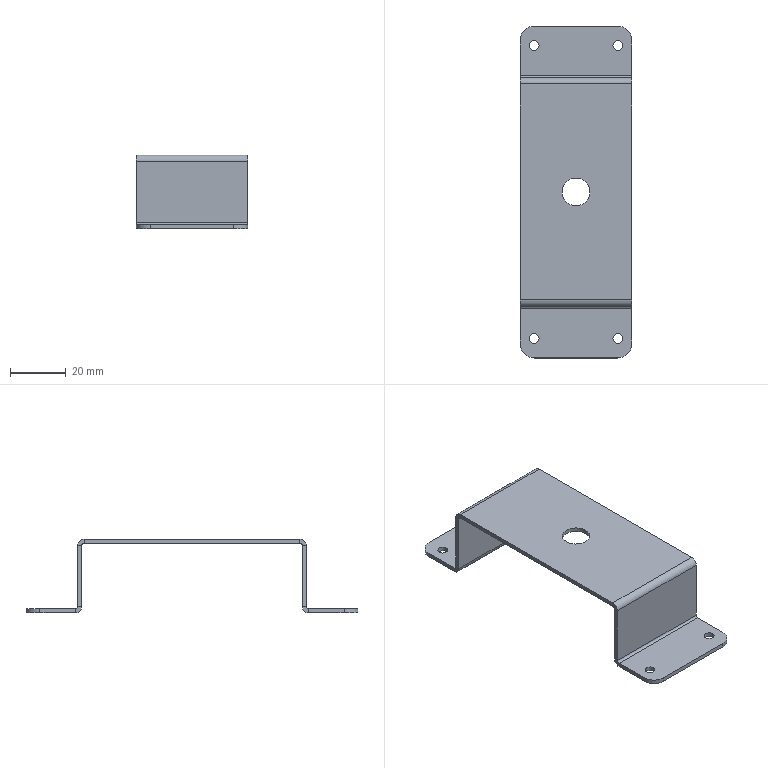Part | SolidWorks | features EdgeFlange 2, ICE 2, Fillet 1, FlatPattern 1, LPattern 1, SMBaseFlange 1, SheetMetal 1 | 1 solid | 52 faces | box 40 x 119 x 26.5 mm | volume 9773 mm3 | plane 30 | cylinder 22 | commonest cylinder face diameters 3.5 x8 10 x6 1.6 x4 4.6 x4
STEP:
#1=CARTESIAN_POINT('',(13.25,52.5,-26.5));
#2=VERTEX_POINT('',#1);
#3=CARTESIAN_POINT('',(16.75,52.5,-26.5));
#4=VERTEX_POINT('',#3);
#5=CARTESIAN_POINT('',(15.,52.5,-26.5));
#6=DIRECTION('',(0.,0.,1.));
#7=DIRECTION('',(1.,0.,0.));
#8=AXIS2_PLACEMENT_3D('',#5,#6,#7);
#9=CIRCLE('',#8,1.75);
#10=EDGE_CURVE('',#2,#4,#9,.T.);
#11=ORIENTED_EDGE('',*,*,#10,.F.);
#12=CARTESIAN_POINT('',(13.25,52.5,-25.));
#13=VERTEX_POINT('',#12);
#14=CARTESIAN_POINT('',(13.25,52.5,-35.));
#15=DIRECTION('',(0.,0.,1.));
#16=VECTOR('',#15,1000.);
#17=LINE('',#14,#16);
#18=EDGE_CURVE('',#2,#13,#17,.T.);
#19=ORIENTED_EDGE('',*,*,#18,.T.);
#20=CARTESIAN_POINT('',(16.75,52.5,-25.));
#21=VERTEX_POINT('',#20);
#22=CARTESIAN_POINT('',(15.,52.5,-25.));
#23=DIRECTION('',(0.,0.,1.));
#24=DIRECTION('',(1.,0.,0.));
#25=AXIS2_PLACEMENT_3D('',#22,#23,#24);
#26=CIRCLE('',#25,1.75);
#27=EDGE_CURVE('',#13,#21,#26,.T.);
#28=ORIENTED_EDGE('',*,*,#27,.T.);
#29=CARTESIAN_POINT('',(16.75,52.5,-35.));
#30=DIRECTION('',(0.,0.,1.));
#31=VECTOR('',#30,1000.);
#32=LINE('',#29,#31);
#33=EDGE_CURVE('',#4,#21,#32,.T.);
#34=ORIENTED_EDGE('',*,*,#33,.F.);
#35=EDGE_LOOP('',(#11,#19,#28,#34));
#36=FACE_OUTER_BOUND('',#35,.T.);
#37=CARTESIAN_POINT('',(15.,52.5,-35.));
#38=DIRECTION('',(0.,0.,1.));
#39=DIRECTION('',(1.,0.,0.));
#40=AXIS2_PLACEMENT_3D('',#37,#38,#39);
#41=CYLINDRICAL_SURFACE('',#40,1.75);
#42=ADVANCED_FACE('',(#36),#41,.F.);
#43=CARTESIAN_POINT('',(-16.75,-52.5,-26.5));
#44=VERTEX_POINT('',#43);
#45=CARTESIAN_POINT('',(-13.25,-52.5,-26.5));
#46=VERTEX_POINT('',#45);
#47=CARTESIAN_POINT('',(-15.,-52.5,-26.5));
#48=DIRECTION('',(0.,0.,1.));
#49=DIRECTION('',(1.,0.,0.));
#50=AXIS2_PLACEMENT_3D('',#47,#48,#49);
#51=CIRCLE('',#50,1.75);
#52=EDGE_CURVE('',#44,#46,#51,.T.);
#53=ORIENTED_EDGE('',*,*,#52,.F.);
#54=CARTESIAN_POINT('',(-16.75,-52.5,-25.));
#55=VERTEX_POINT('',#54);
#56=CARTESIAN_POINT('',(-16.75,-52.5,-35.));
#57=DIRECTION('',(0.,0.,1.));
#58=VECTOR('',#57,1000.);
#59=LINE('',#56,#58);
#60=EDGE_CURVE('',#44,#55,#59,.T.);
#61=ORIENTED_EDGE('',*,*,#60,.T.);
#62=CARTESIAN_POINT('',(-13.25,-52.5,-25.));
#63=VERTEX_POINT('',#62);
#64=CARTESIAN_POINT('',(-15.,-52.5,-25.));
#65=DIRECTION('',(0.,0.,1.));
#66=DIRECTION('',(1.,0.,0.));
#67=AXIS2_PLACEMENT_3D('',#64,#65,#66);
#68=CIRCLE('',#67,1.75);
#69=EDGE_CURVE('',#55,#63,#68,.T.);
#70=ORIENTED_EDGE('',*,*,#69,.T.);
#71=CARTESIAN_POINT('',(-13.25,-52.5,-35.));
#72=DIRECTION('',(0.,0.,1.));
#73=VECTOR('',#72,1000.);
#74=LINE('',#71,#73);
#75=EDGE_CURVE('',#46,#63,#74,.T.);
#76=ORIENTED_EDGE('',*,*,#75,.F.);
#77=EDGE_LOOP('',(#53,#61,#70,#76));
#78=FACE_OUTER_BOUND('',#77,.T.);
#79=CARTESIAN_POINT('',(-15.,-52.5,-35.));
#80=DIRECTION('',(0.,0.,1.));
#81=DIRECTION('',(1.,0.,0.));
#82=AXIS2_PLACEMENT_3D('',#79,#80,#81);
#83=CYLINDRICAL_SURFACE('',#82,1.75);
#84=ADVANCED_FACE('',(#78),#83,.F.);
#85=CARTESIAN_POINT('',(13.25,-52.5,-26.5));
#86=VERTEX_POINT('',#85);
#87=CARTESIAN_POINT('',(16.75,-52.5,-26.5));
#88=VERTEX_POINT('',#87);
#89=CARTESIAN_POINT('',(15.,-52.5,-26.5));
#90=DIRECTION('',(0.,0.,1.));
#91=DIRECTION('',(1.,0.,0.));
#92=AXIS2_PLACEMENT_3D('',#89,#90,#91);
#93=CIRCLE('',#92,1.75);
#94=EDGE_CURVE('',#86,#88,#93,.T.);
#95=ORIENTED_EDGE('',*,*,#94,.F.);
#96=CARTESIAN_POINT('',(13.25,-52.5,-25.));
#97=VERTEX_POINT('',#96);
#98=CARTESIAN_POINT('',(13.25,-52.5,-35.));
#99=DIRECTION('',(0.,0.,1.));
#100=VECTOR('',#99,1000.);
#101=LINE('',#98,#100);
#102=EDGE_CURVE('',#86,#97,#101,.T.);
#103=ORIENTED_EDGE('',*,*,#102,.T.);
#104=CARTESIAN_POINT('',(16.75,-52.5,-25.));
#105=VERTEX_POINT('',#104);
#106=CARTESIAN_POINT('',(15.,-52.5,-25.));
#107=DIRECTION('',(0.,0.,1.));
#108=DIRECTION('',(1.,0.,0.));
#109=AXIS2_PLACEMENT_3D('',#106,#107,#108);
#110=CIRCLE('',#109,1.75);
#111=EDGE_CURVE('',#97,#105,#110,.T.);
#112=ORIENTED_EDGE('',*,*,#111,.T.);
#113=CARTESIAN_POINT('',(16.75,-52.5,-35.));
#114=DIRECTION('',(0.,0.,1.));
#115=VECTOR('',#114,1000.);
#116=LINE('',#113,#115);
#117=EDGE_CURVE('',#88,#105,#116,.T.);
#118=ORIENTED_EDGE('',*,*,#117,.F.);
#119=EDGE_LOOP('',(#95,#103,#112,#118));
#120=FACE_OUTER_BOUND('',#119,.T.);
#121=CARTESIAN_POINT('',(15.,-52.5,-35.));
#122=DIRECTION('',(0.,0.,1.));
#123=DIRECTION('',(1.,0.,0.));
#124=AXIS2_PLACEMENT_3D('',#121,#122,#123);
#125=CYLINDRICAL_SURFACE('',#124,1.75);
#126=ADVANCED_FACE('',(#120),#125,.F.);
#127=CARTESIAN_POINT('',(-16.75,52.5,-26.5));
#128=VERTEX_POINT('',#127);
#129=CARTESIAN_POINT('',(-13.25,52.5,-26.5));
#130=VERTEX_POINT('',#129);
#131=CARTESIAN_POINT('',(-15.,52.5,-26.5));
#132=DIRECTION('',(0.,0.,1.));
#133=DIRECTION('',(1.,0.,0.));
#134=AXIS2_PLACEMENT_3D('',#131,#132,#133);
#135=CIRCLE('',#134,1.75);
#136=EDGE_CURVE('',#128,#130,#135,.T.);
#137=ORIENTED_EDGE('',*,*,#136,.F.);
#138=CARTESIAN_POINT('',(-16.75,52.5,-25.));
#139=VERTEX_POINT('',#138);
#140=CARTESIAN_POINT('',(-16.75,52.5,-35.));
#141=DIRECTION('',(0.,0.,1.));
#142=VECTOR('',#141,1000.);
#143=LINE('',#140,#142);
#144=EDGE_CURVE('',#128,#139,#143,.T.);
#145=ORIENTED_EDGE('',*,*,#144,.T.);
#146=CARTESIAN_POINT('',(-13.25,52.5,-25.));
#147=VERTEX_POINT('',#146);
#148=CARTESIAN_POINT('',(-15.,52.5,-25.));
#149=DIRECTION('',(0.,0.,1.));
#150=DIRECTION('',(1.,0.,0.));
#151=AXIS2_PLACEMENT_3D('',#148,#149,#150);
#152=CIRCLE('',#151,1.75);
#153=EDGE_CURVE('',#139,#147,#152,.T.);
#154=ORIENTED_EDGE('',*,*,#153,.T.);
#155=CARTESIAN_POINT('',(-13.25,52.5,-35.));
#156=DIRECTION('',(0.,0.,1.));
#157=VECTOR('',#156,1000.);
#158=LINE('',#155,#157);
#159=EDGE_CURVE('',#130,#147,#158,.T.);
#160=ORIENTED_EDGE('',*,*,#159,.F.);
#161=EDGE_LOOP('',(#137,#145,#154,#160));
#162=FACE_OUTER_BOUND('',#161,.T.);
#163=CARTESIAN_POINT('',(-15.,52.5,-35.));
#164=DIRECTION('',(0.,0.,1.));
#165=DIRECTION('',(1.,0.,0.));
#166=AXIS2_PLACEMENT_3D('',#163,#164,#165);
#167=CYLINDRICAL_SURFACE('',#166,1.75);
#168=ADVANCED_FACE('',(#162),#167,.F.);
#169=CARTESIAN_POINT('',(5.,0.,-1.5));
#170=VERTEX_POINT('',#169);
#171=CARTESIAN_POINT('',(-5.,0.,-1.5));
#172=VERTEX_POINT('',#171);
#173=CARTESIAN_POINT('',(0.,0.,-1.5));
#174=DIRECTION('',(0.,0.,-1.));
#175=DIRECTION('',(-1.,0.,0.));
#176=AXIS2_PLACEMENT_3D('',#173,#174,#175);
#177=CIRCLE('',#176,5.);
#178=EDGE_CURVE('',#170,#172,#177,.T.);
#179=ORIENTED_EDGE('',*,*,#178,.T.);
#180=CARTESIAN_POINT('',(-5.,0.,0.));
#181=VERTEX_POINT('',#180);
#182=CARTESIAN_POINT('',(-5.,0.,-10.));
#183=DIRECTION('',(0.,0.,1.));
#184=VECTOR('',#183,1000.);
#185=LINE('',#182,#184);
#186=EDGE_CURVE('',#172,#181,#185,.T.);
#187=ORIENTED_EDGE('',*,*,#186,.T.);
#188=CARTESIAN_POINT('',(5.,0.,0.));
#189=VERTEX_POINT('',#188);
#190=CARTESIAN_POINT('',(0.,0.,0.));
#191=DIRECTION('',(0.,0.,1.));
#192=DIRECTION('',(1.,0.,0.));
#193=AXIS2_PLACEMENT_3D('',#190,#191,#192);
#194=CIRCLE('',#193,5.);
#195=EDGE_CURVE('',#181,#189,#194,.T.);
#196=ORIENTED_EDGE('',*,*,#195,.T.);
#197=CARTESIAN_POINT('',(5.,0.,-10.));
#198=DIRECTION('',(0.,0.,1.));
#199=VECTOR('',#198,1000.);
#200=LINE('',#197,#199);
#201=EDGE_CURVE('',#170,#189,#200,.T.);
#202=ORIENTED_EDGE('',*,*,#201,.F.);
#203=EDGE_LOOP('',(#179,#187,#196,#202));
#204=FACE_OUTER_BOUND('',#203,.T.);
#205=CARTESIAN_POINT('',(0.,0.,-10.));
#206=DIRECTION('',(0.,0.,1.));
#207=DIRECTION('',(1.,0.,0.));
#208=AXIS2_PLACEMENT_3D('',#205,#206,#207);
#209=CYLINDRICAL_SURFACE('',#208,5.);
#210=ADVANCED_FACE('',(#204),#209,.F.);
#211=CARTESIAN_POINT('',(20.,-41.,-2.3));
#212=VERTEX_POINT('',#211);
#213=CARTESIAN_POINT('',(20.,-41.,-24.2));
#214=VERTEX_POINT('',#213);
#215=CARTESIAN_POINT('',(20.,-41.,-1.5));
#216=DIRECTION('',(0.,0.,-1.));
#217=VECTOR('',#216,1000.);
#218=LINE('',#215,#217);
#219=EDGE_CURVE('',#212,#214,#218,.T.);
#220=ORIENTED_EDGE('',*,*,#219,.T.);
#221=CARTESIAN_POINT('',(20.,-39.5,-24.2));
#222=VERTEX_POINT('',#221);
#223=CARTESIAN_POINT('',(20.,-41.,-24.2));
#224=DIRECTION('',(0.,1.,0.));
#225=VECTOR('',#224,1000.);
#226=LINE('',#223,#225);
#227=EDGE_CURVE('',#214,#222,#226,.T.);
#228=ORIENTED_EDGE('',*,*,#227,.T.);
#229=CARTESIAN_POINT('',(20.,-39.5,-2.3));
#230=VERTEX_POINT('',#229);
#231=CARTESIAN_POINT('',(20.,-39.5,0.));
#232=DIRECTION('',(0.,0.,-1.));
#233=VECTOR('',#232,1000.);
#234=LINE('',#231,#233);
#235=EDGE_CURVE('',#230,#222,#234,.T.);
#236=ORIENTED_EDGE('',*,*,#235,.F.);
#237=CARTESIAN_POINT('',(20.,-41.,-2.3));
#238=DIRECTION('',(0.,-1.,0.));
#239=VECTOR('',#238,1000.);
#240=LINE('',#237,#239);
#241=EDGE_CURVE('',#230,#212,#240,.T.);
#242=ORIENTED_EDGE('',*,*,#241,.T.);
#243=EDGE_LOOP('',(#220,#228,#236,#242));
#244=FACE_OUTER_BOUND('',#243,.T.);
#245=CARTESIAN_POINT('',(20.,-41.,-1.5));
#246=DIRECTION('',(1.,0.,0.));
#247=DIRECTION('',(0.,0.,-1.));
#248=AXIS2_PLACEMENT_3D('',#245,#246,#247);
#249=PLANE('',#248);
#250=ADVANCED_FACE('',(#244),#249,.T.);
#251=CARTESIAN_POINT('',(-20.,-41.,-24.2));
#252=VERTEX_POINT('',#251);
#253=CARTESIAN_POINT('',(20.,-41.,-24.2));
#254=DIRECTION('',(-1.,0.,0.));
#255=VECTOR('',#254,1000.);
#256=LINE('',#253,#255);
#257=EDGE_CURVE('',#214,#252,#256,.T.);
#258=ORIENTED_EDGE('',*,*,#257,.F.);
#259=ORIENTED_EDGE('',*,*,#219,.F.);
#260=CARTESIAN_POINT('',(-20.,-41.,-2.3));
#261=VERTEX_POINT('',#260);
#262=CARTESIAN_POINT('',(20.,-41.,-2.3));
#263=DIRECTION('',(1.,0.,0.));
#264=VECTOR('',#263,1000.);
#265=LINE('',#262,#264);
#266=EDGE_CURVE('',#261,#212,#265,.T.);
#267=ORIENTED_EDGE('',*,*,#266,.F.);
#268=CARTESIAN_POINT('',(-20.,-41.,-25.));
#269=DIRECTION('',(0.,0.,1.));
#270=VECTOR('',#269,1000.);
#271=LINE('',#268,#270);
#272=EDGE_CURVE('',#252,#261,#271,.T.);
#273=ORIENTED_EDGE('',*,*,#272,.F.);
#274=EDGE_LOOP('',(#258,#259,#267,#273));
#275=FACE_OUTER_BOUND('',#274,.T.);
#276=CARTESIAN_POINT('',(0.,-41.,0.));
#277=DIRECTION('',(0.,1.,0.));
#278=DIRECTION('',(0.,0.,1.));
#279=AXIS2_PLACEMENT_3D('',#276,#277,#278);
#280=PLANE('',#279);
#281=ADVANCED_FACE('',(#275),#280,.F.);
#282=ORIENTED_EDGE('',*,*,#235,.T.);
#283=CARTESIAN_POINT('',(-20.,-39.5,-24.2));
#284=VERTEX_POINT('',#283);
#285=CARTESIAN_POINT('',(20.,-39.5,-24.2));
#286=DIRECTION('',(-1.,0.,0.));
#287=VECTOR('',#286,1000.);
#288=LINE('',#285,#287);
#289=EDGE_CURVE('',#222,#284,#288,.T.);
#290=ORIENTED_EDGE('',*,*,#289,.T.);
#291=CARTESIAN_POINT('',(-20.,-39.5,-2.3));
#292=VERTEX_POINT('',#291);
#293=CARTESIAN_POINT('',(-20.,-39.5,0.));
#294=DIRECTION('',(0.,0.,1.));
#295=VECTOR('',#294,1000.);
#296=LINE('',#293,#295);
#297=EDGE_CURVE('',#284,#292,#296,.T.);
#298=ORIENTED_EDGE('',*,*,#297,.T.);
#299=CARTESIAN_POINT('',(20.,-39.5,-2.3));
#300=DIRECTION('',(-1.,0.,0.));
#301=VECTOR('',#300,1000.);
#302=LINE('',#299,#301);
#303=EDGE_CURVE('',#230,#292,#302,.T.);
#304=ORIENTED_EDGE('',*,*,#303,.F.);
#305=EDGE_LOOP('',(#282,#290,#298,#304));
#306=FACE_OUTER_BOUND('',#305,.T.);
#307=CARTESIAN_POINT('',(0.,-39.5,0.));
#308=DIRECTION('',(0.,1.,0.));
#309=DIRECTION('',(0.,0.,1.));
#310=AXIS2_PLACEMENT_3D('',#307,#308,#309);
#311=PLANE('',#310);
#312=ADVANCED_FACE('',(#306),#311,.T.);
#313=CARTESIAN_POINT('',(-20.,41.,-2.3));
#314=VERTEX_POINT('',#313);
#315=CARTESIAN_POINT('',(-20.,41.,-24.2));
#316=VERTEX_POINT('',#315);
#317=CARTESIAN_POINT('',(-20.,41.,-25.));
#318=DIRECTION('',(0.,0.,-1.));
#319=VECTOR('',#318,1000.);
#320=LINE('',#317,#319);
#321=EDGE_CURVE('',#314,#316,#320,.T.);
#322=ORIENTED_EDGE('',*,*,#321,.T.);
#323=CARTESIAN_POINT('',(-20.,39.5,-24.2));
#324=VERTEX_POINT('',#323);
#325=CARTESIAN_POINT('',(-20.,41.,-24.2));
#326=DIRECTION('',(0.,-1.,0.));
#327=VECTOR('',#326,1000.);
#328=LINE('',#325,#327);
#329=EDGE_CURVE('',#316,#324,#328,.T.);
#330=ORIENTED_EDGE('',*,*,#329,.T.);
#331=CARTESIAN_POINT('',(-20.,39.5,-2.3));
#332=VERTEX_POINT('',#331);
#333=CARTESIAN_POINT('',(-20.,39.5,0.));
#334=DIRECTION('',(0.,0.,-1.));
#335=VECTOR('',#334,1000.);
#336=LINE('',#333,#335);
#337=EDGE_CURVE('',#332,#324,#336,.T.);
#338=ORIENTED_EDGE('',*,*,#337,.F.);
#339=CARTESIAN_POINT('',(-20.,41.,-2.3));
#340=DIRECTION('',(0.,1.,0.));
#341=VECTOR('',#340,1000.);
#342=LINE('',#339,#341);
#343=EDGE_CURVE('',#332,#314,#342,.T.);
#344=ORIENTED_EDGE('',*,*,#343,.T.);
#345=EDGE_LOOP('',(#322,#330,#338,#344));
#346=FACE_OUTER_BOUND('',#345,.T.);
#347=CARTESIAN_POINT('',(-20.,41.,-25.));
#348=DIRECTION('',(-1.,0.,0.));
#349=DIRECTION('',(0.,0.,1.));
#350=AXIS2_PLACEMENT_3D('',#347,#348,#349);
#351=PLANE('',#350);
#352=ADVANCED_FACE('',(#346),#351,.T.);
#353=CARTESIAN_POINT('',(20.,41.,-24.2));
#354=VERTEX_POINT('',#353);
#355=CARTESIAN_POINT('',(20.,41.,-2.3));
#356=VERTEX_POINT('',#355);
#357=CARTESIAN_POINT('',(20.,41.,-1.5));
#358=DIRECTION('',(0.,0.,1.));
#359=VECTOR('',#358,1000.);
#360=LINE('',#357,#359);
#361=EDGE_CURVE('',#354,#356,#360,.T.);
#362=ORIENTED_EDGE('',*,*,#361,.F.);
#363=CARTESIAN_POINT('',(-20.,41.,-24.2));
#364=DIRECTION('',(1.,0.,0.));
#365=VECTOR('',#364,1000.);
#366=LINE('',#363,#365);
#367=EDGE_CURVE('',#316,#354,#366,.T.);
#368=ORIENTED_EDGE('',*,*,#367,.F.);
#369=ORIENTED_EDGE('',*,*,#321,.F.);
#370=CARTESIAN_POINT('',(0.,41.,-2.3));
#371=DIRECTION('',(1.,0.,0.));
#372=VECTOR('',#371,1000.);
#373=LINE('',#370,#372);
#374=EDGE_CURVE('',#314,#356,#373,.T.);
#375=ORIENTED_EDGE('',*,*,#374,.T.);
#376=EDGE_LOOP('',(#362,#368,#369,#375));
#377=FACE_OUTER_BOUND('',#376,.T.);
#378=CARTESIAN_POINT('',(0.,41.,0.));
#379=DIRECTION('',(0.,1.,0.));
#380=DIRECTION('',(0.,0.,1.));
#381=AXIS2_PLACEMENT_3D('',#378,#379,#380);
#382=PLANE('',#381);
#383=ADVANCED_FACE('',(#377),#382,.T.);
#384=CARTESIAN_POINT('',(20.,39.5,-24.2));
#385=VERTEX_POINT('',#384);
#386=CARTESIAN_POINT('',(-20.,39.5,-24.2));
#387=DIRECTION('',(1.,0.,0.));
#388=VECTOR('',#387,1000.);
#389=LINE('',#386,#388);
#390=EDGE_CURVE('',#324,#385,#389,.T.);
#391=ORIENTED_EDGE('',*,*,#390,.T.);
#392=CARTESIAN_POINT('',(20.,39.5,-2.3));
#393=VERTEX_POINT('',#392);
#394=CARTESIAN_POINT('',(20.,39.5,0.));
#395=DIRECTION('',(0.,0.,1.));
#396=VECTOR('',#395,1000.);
#397=LINE('',#394,#396);
#398=EDGE_CURVE('',#385,#393,#397,.T.);
#399=ORIENTED_EDGE('',*,*,#398,.T.);
#400=CARTESIAN_POINT('',(-20.,39.5,-2.3));
#401=DIRECTION('',(1.,0.,0.));
#402=VECTOR('',#401,1000.);
#403=LINE('',#400,#402);
#404=EDGE_CURVE('',#332,#393,#403,.T.);
#405=ORIENTED_EDGE('',*,*,#404,.F.);
#406=ORIENTED_EDGE('',*,*,#337,.T.);
#407=EDGE_LOOP('',(#391,#399,#405,#406));
#408=FACE_OUTER_BOUND('',#407,.T.);
#409=CARTESIAN_POINT('',(0.,39.5,0.));
#410=DIRECTION('',(0.,1.,0.));
#411=DIRECTION('',(0.,0.,1.));
#412=AXIS2_PLACEMENT_3D('',#409,#410,#411);
#413=PLANE('',#412);
#414=ADVANCED_FACE('',(#408),#413,.F.);
#415=ORIENTED_EDGE('',*,*,#178,.F.);
#416=CARTESIAN_POINT('',(0.,0.,-1.5));
#417=DIRECTION('',(0.,0.,-1.));
#418=DIRECTION('',(-1.,0.,0.));
#419=AXIS2_PLACEMENT_3D('',#416,#417,#418);
#420=CIRCLE('',#419,5.);
#421=EDGE_CURVE('',#172,#170,#420,.T.);
#422=ORIENTED_EDGE('',*,*,#421,.F.);
#423=EDGE_LOOP('',(#415,#422));
#424=FACE_BOUND('',#423,.T.);
#425=CARTESIAN_POINT('',(20.,-38.7,-1.5));
#426=VERTEX_POINT('',#425);
#427=CARTESIAN_POINT('',(20.,38.7,-1.5));
#428=VERTEX_POINT('',#427);
#429=CARTESIAN_POINT('',(20.,-41.,-1.5));
#430=DIRECTION('',(0.,1.,0.));
#431=VECTOR('',#430,1000.);
#432=LINE('',#429,#431);
#433=EDGE_CURVE('',#426,#428,#432,.T.);
#434=ORIENTED_EDGE('',*,*,#433,.F.);
#435=CARTESIAN_POINT('',(-20.,-38.7,-1.5));
#436=VERTEX_POINT('',#435);
#437=CARTESIAN_POINT('',(-20.,-38.7,-1.5));
#438=DIRECTION('',(1.,0.,0.));
#439=VECTOR('',#438,1000.);
#440=LINE('',#437,#439);
#441=EDGE_CURVE('',#436,#426,#440,.T.);
#442=ORIENTED_EDGE('',*,*,#441,.F.);
#443=CARTESIAN_POINT('',(-20.,38.7,-1.5));
#444=VERTEX_POINT('',#443);
#445=CARTESIAN_POINT('',(-20.,-41.,-1.5));
#446=DIRECTION('',(0.,-1.,0.));
#447=VECTOR('',#446,1000.);
#448=LINE('',#445,#447);
#449=EDGE_CURVE('',#444,#436,#448,.T.);
#450=ORIENTED_EDGE('',*,*,#449,.F.);
#451=CARTESIAN_POINT('',(20.,38.7,-1.5));
#452=DIRECTION('',(-1.,0.,0.));
#453=VECTOR('',#452,1000.);
#454=LINE('',#451,#453);
#455=EDGE_CURVE('',#428,#444,#454,.T.);
#456=ORIENTED_EDGE('',*,*,#455,.F.);
#457=EDGE_LOOP('',(#434,#442,#450,#456));
#458=FACE_OUTER_BOUND('',#457,.T.);
#459=CARTESIAN_POINT('',(0.,0.,-1.5));
#460=DIRECTION('',(0.,0.,-1.));
#461=DIRECTION('',(-1.,0.,0.));
#462=AXIS2_PLACEMENT_3D('',#459,#460,#461);
#463=PLANE('',#462);
#464=ADVANCED_FACE('',(#424,#458),#463,.T.);
#465=CARTESIAN_POINT('',(0.,0.,0.));
#466=DIRECTION('',(0.,0.,1.));
#467=DIRECTION('',(1.,0.,0.));
#468=AXIS2_PLACEMENT_3D('',#465,#466,#467);
#469=CIRCLE('',#468,5.);
#470=EDGE_CURVE('',#189,#181,#469,.T.);
#471=ORIENTED_EDGE('',*,*,#470,.F.);
#472=ORIENTED_EDGE('',*,*,#195,.F.);
#473=EDGE_LOOP('',(#471,#472));
#474=FACE_BOUND('',#473,.T.);
#475=CARTESIAN_POINT('',(-20.,-38.7,0.));
#476=VERTEX_POINT('',#475);
#477=CARTESIAN_POINT('',(20.,-38.7,0.));
#478=VERTEX_POINT('',#477);
#479=CARTESIAN_POINT('',(-20.,-38.7,0.));
#480=DIRECTION('',(1.,0.,0.));
#481=VECTOR('',#480,1000.);
#482=LINE('',#479,#481);
#483=EDGE_CURVE('',#476,#478,#482,.T.);
#484=ORIENTED_EDGE('',*,*,#483,.T.);
#485=CARTESIAN_POINT('',(20.,38.7,0.));
#486=VERTEX_POINT('',#485);
#487=CARTESIAN_POINT('',(20.,-41.,0.));
#488=DIRECTION('',(0.,1.,0.));
#489=VECTOR('',#488,1000.);
#490=LINE('',#487,#489);
#491=EDGE_CURVE('',#478,#486,#490,.T.);
#492=ORIENTED_EDGE('',*,*,#491,.T.);
#493=CARTESIAN_POINT('',(-20.,38.7,0.));
#494=VERTEX_POINT('',#493);
#495=CARTESIAN_POINT('',(20.,38.7,0.));
#496=DIRECTION('',(-1.,0.,0.));
#497=VECTOR('',#496,1000.);
#498=LINE('',#495,#497);
#499=EDGE_CURVE('',#486,#494,#498,.T.);
#500=ORIENTED_EDGE('',*,*,#499,.T.);
#501=CARTESIAN_POINT('',(-20.,-41.,0.));
#502=DIRECTION('',(0.,-1.,0.));
#503=VECTOR('',#502,1000.);
#504=LINE('',#501,#503);
#505=EDGE_CURVE('',#494,#476,#504,.T.);
#506=ORIENTED_EDGE('',*,*,#505,.T.);
#507=EDGE_LOOP('',(#484,#492,#500,#506));
#508=FACE_OUTER_BOUND('',#507,.T.);
#509=CARTESIAN_POINT('',(0.,0.,0.));
#510=DIRECTION('',(0.,0.,-1.));
#511=DIRECTION('',(-1.,0.,0.));
#512=AXIS2_PLACEMENT_3D('',#509,#510,#511);
#513=PLANE('',#512);
#514=ADVANCED_FACE('',(#474,#508),#513,.F.);
#515=ORIENTED_EDGE('',*,*,#449,.T.);
#516=CARTESIAN_POINT('',(-20.,-38.7,-1.5));
#517=DIRECTION('',(0.,0.,1.));
#518=VECTOR('',#517,1000.);
#519=LINE('',#516,#518);
#520=EDGE_CURVE('',#436,#476,#519,.T.);
#521=ORIENTED_EDGE('',*,*,#520,.T.);
#522=ORIENTED_EDGE('',*,*,#505,.F.);
#523=CARTESIAN_POINT('',(-20.,38.7,-1.5));
#524=DIRECTION('',(0.,0.,1.));
#525=VECTOR('',#524,1000.);
#526=LINE('',#523,#525);
#527=EDGE_CURVE('',#444,#494,#526,.T.);
#528=ORIENTED_EDGE('',*,*,#527,.F.);
#529=EDGE_LOOP('',(#515,#521,#522,#528));
#530=FACE_OUTER_BOUND('',#529,.T.);
#531=CARTESIAN_POINT('',(-20.,-41.,-1.5));
#532=DIRECTION('',(-1.,0.,0.));
#533=DIRECTION('',(0.,0.,1.));
#534=AXIS2_PLACEMENT_3D('',#531,#532,#533);
#535=PLANE('',#534);
#536=ADVANCED_FACE('',(#530),#535,.T.);
#537=CARTESIAN_POINT('',(20.,-38.7,-1.5));
#538=DIRECTION('',(0.,0.,1.));
#539=VECTOR('',#538,1000.);
#540=LINE('',#537,#539);
#541=EDGE_CURVE('',#426,#478,#540,.T.);
#542=ORIENTED_EDGE('',*,*,#541,.F.);
#543=ORIENTED_EDGE('',*,*,#433,.T.);
#544=CARTESIAN_POINT('',(20.,38.7,-1.5));
#545=DIRECTION('',(0.,0.,1.));
#546=VECTOR('',#545,1000.);
#547=LINE('',#544,#546);
#548=EDGE_CURVE('',#428,#486,#547,.T.);
#549=ORIENTED_EDGE('',*,*,#548,.T.);
#550=ORIENTED_EDGE('',*,*,#491,.F.);
#551=EDGE_LOOP('',(#542,#543,#549,#550));
#552=FACE_OUTER_BOUND('',#551,.T.);
#553=CARTESIAN_POINT('',(20.,-41.,-1.5));
#554=DIRECTION('',(1.,0.,0.));
#555=DIRECTION('',(0.,0.,-1.));
#556=AXIS2_PLACEMENT_3D('',#553,#554,#555);
#557=PLANE('',#556);
#558=ADVANCED_FACE('',(#552),#557,.T.);
#559=ORIENTED_EDGE('',*,*,#343,.F.);
#560=CARTESIAN_POINT('',(-20.,38.7,-2.3));
#561=DIRECTION('',(-1.,0.,0.));
#562=DIRECTION('',(0.,0.,-1.));
#563=AXIS2_PLACEMENT_3D('',#560,#561,#562);
#564=CIRCLE('',#563,0.8);
#565=EDGE_CURVE('',#444,#332,#564,.T.);
#566=ORIENTED_EDGE('',*,*,#565,.F.);
#567=ORIENTED_EDGE('',*,*,#527,.T.);
#568=CARTESIAN_POINT('',(-20.,38.7,-2.3));
#569=DIRECTION('',(-1.,0.,0.));
#570=DIRECTION('',(0.,0.,-1.));
#571=AXIS2_PLACEMENT_3D('',#568,#569,#570);
#572=CIRCLE('',#571,2.3);
#573=EDGE_CURVE('',#494,#314,#572,.T.);
#574=ORIENTED_EDGE('',*,*,#573,.T.);
#575=EDGE_LOOP('',(#559,#566,#567,#574));
#576=FACE_OUTER_BOUND('',#575,.T.);
#577=CARTESIAN_POINT('',(-20.,38.7,-2.3));
#578=DIRECTION('',(-1.,0.,0.));
#579=DIRECTION('',(0.,0.,1.));
#580=AXIS2_PLACEMENT_3D('',#577,#578,#579);
#581=PLANE('',#580);
#582=ADVANCED_FACE('',(#576),#581,.T.);
#583=CARTESIAN_POINT('',(20.,38.7,-2.3));
#584=DIRECTION('',(1.,0.,0.));
#585=DIRECTION('',(0.,0.,-1.));
#586=AXIS2_PLACEMENT_3D('',#583,#584,#585);
#587=CIRCLE('',#586,0.8);
#588=EDGE_CURVE('',#393,#428,#587,.T.);
#589=ORIENTED_EDGE('',*,*,#588,.F.);
#590=CARTESIAN_POINT('',(20.,39.5,-2.3));
#591=DIRECTION('',(0.,1.,0.));
#592=VECTOR('',#591,1000.);
#593=LINE('',#590,#592);
#594=EDGE_CURVE('',#393,#356,#593,.T.);
#595=ORIENTED_EDGE('',*,*,#594,.T.);
#596=CARTESIAN_POINT('',(20.,38.7,-2.3));
#597=DIRECTION('',(1.,0.,0.));
#598=DIRECTION('',(0.,0.,-1.));
#599=AXIS2_PLACEMENT_3D('',#596,#597,#598);
#600=CIRCLE('',#599,2.3);
#601=EDGE_CURVE('',#356,#486,#600,.T.);
#602=ORIENTED_EDGE('',*,*,#601,.T.);
#603=ORIENTED_EDGE('',*,*,#548,.F.);
#604=EDGE_LOOP('',(#589,#595,#602,#603));
#605=FACE_OUTER_BOUND('',#604,.T.);
#606=CARTESIAN_POINT('',(20.,38.7,-2.3));
#607=DIRECTION('',(-1.,0.,0.));
#608=DIRECTION('',(0.,0.,1.));
#609=AXIS2_PLACEMENT_3D('',#606,#607,#608);
#610=PLANE('',#609);
#611=ADVANCED_FACE('',(#605),#610,.F.);
#612=ORIENTED_EDGE('',*,*,#499,.F.);
#613=ORIENTED_EDGE('',*,*,#601,.F.);
#614=ORIENTED_EDGE('',*,*,#374,.F.);
#615=ORIENTED_EDGE('',*,*,#573,.F.);
#616=EDGE_LOOP('',(#612,#613,#614,#615));
#617=FACE_OUTER_BOUND('',#616,.T.);
#618=CARTESIAN_POINT('',(20.,38.7,-2.3));
#619=DIRECTION('',(1.,0.,0.));
#620=DIRECTION('',(0.,1.,0.));
#621=AXIS2_PLACEMENT_3D('',#618,#619,#620);
#622=CYLINDRICAL_SURFACE('',#621,2.3);
#623=ADVANCED_FACE('',(#617),#622,.T.);
#624=ORIENTED_EDGE('',*,*,#455,.T.);
#625=ORIENTED_EDGE('',*,*,#565,.T.);
#626=ORIENTED_EDGE('',*,*,#404,.T.);
#627=ORIENTED_EDGE('',*,*,#588,.T.);
#628=EDGE_LOOP('',(#624,#625,#626,#627));
#629=FACE_OUTER_BOUND('',#628,.T.);
#630=CARTESIAN_POINT('',(20.,38.7,-2.3));
#631=DIRECTION('',(1.,0.,0.));
#632=DIRECTION('',(0.,1.,0.));
#633=AXIS2_PLACEMENT_3D('',#630,#631,#632);
#634=CYLINDRICAL_SURFACE('',#633,0.8);
#635=ADVANCED_FACE('',(#629),#634,.F.);
#636=CARTESIAN_POINT('',(20.,41.,-24.2));
#637=DIRECTION('',(0.,-1.,0.));
#638=VECTOR('',#637,1000.);
#639=LINE('',#636,#638);
#640=EDGE_CURVE('',#354,#385,#639,.T.);
#641=ORIENTED_EDGE('',*,*,#640,.F.);
#642=ORIENTED_EDGE('',*,*,#361,.T.);
#643=ORIENTED_EDGE('',*,*,#594,.F.);
#644=ORIENTED_EDGE('',*,*,#398,.F.);
#645=EDGE_LOOP('',(#641,#642,#643,#644));
#646=FACE_OUTER_BOUND('',#645,.T.);
#647=CARTESIAN_POINT('',(20.,41.,-1.5));
#648=DIRECTION('',(1.,0.,0.));
#649=DIRECTION('',(0.,0.,-1.));
#650=AXIS2_PLACEMENT_3D('',#647,#648,#649);
#651=PLANE('',#650);
#652=ADVANCED_FACE('',(#646),#651,.T.);
#653=ORIENTED_EDGE('',*,*,#241,.F.);
#654=CARTESIAN_POINT('',(20.,-38.7,-2.3));
#655=DIRECTION('',(1.,0.,0.));
#656=DIRECTION('',(0.,0.,1.));
#657=AXIS2_PLACEMENT_3D('',#654,#655,#656);
#658=CIRCLE('',#657,0.8);
#659=EDGE_CURVE('',#426,#230,#658,.T.);
#660=ORIENTED_EDGE('',*,*,#659,.F.);
#661=ORIENTED_EDGE('',*,*,#541,.T.);
#662=CARTESIAN_POINT('',(20.,-38.7,-2.3));
#663=DIRECTION('',(1.,0.,0.));
#664=DIRECTION('',(0.,0.,1.));
#665=AXIS2_PLACEMENT_3D('',#662,#663,#664);
#666=CIRCLE('',#665,2.3);
#667=EDGE_CURVE('',#478,#212,#666,.T.);
#668=ORIENTED_EDGE('',*,*,#667,.T.);
#669=EDGE_LOOP('',(#653,#660,#661,#668));
#670=FACE_OUTER_BOUND('',#669,.T.);
#671=CARTESIAN_POINT('',(20.,-38.7,-2.3));
#672=DIRECTION('',(1.,0.,0.));
#673=DIRECTION('',(0.,0.,-1.));
#674=AXIS2_PLACEMENT_3D('',#671,#672,#673);
#675=PLANE('',#674);
#676=ADVANCED_FACE('',(#670),#675,.T.);
#677=CARTESIAN_POINT('',(-20.,-38.7,-2.3));
#678=DIRECTION('',(-1.,0.,0.));
#679=DIRECTION('',(0.,0.,1.));
#680=AXIS2_PLACEMENT_3D('',#677,#678,#679);
#681=CIRCLE('',#680,0.8);
#682=EDGE_CURVE('',#292,#436,#681,.T.);
#683=ORIENTED_EDGE('',*,*,#682,.F.);
#684=CARTESIAN_POINT('',(-20.,-39.5,-2.3));
#685=DIRECTION('',(0.,-1.,0.));
#686=VECTOR('',#685,1000.);
#687=LINE('',#684,#686);
#688=EDGE_CURVE('',#292,#261,#687,.T.);
#689=ORIENTED_EDGE('',*,*,#688,.T.);
#690=CARTESIAN_POINT('',(-20.,-38.7,-2.3));
#691=DIRECTION('',(-1.,0.,0.));
#692=DIRECTION('',(0.,0.,1.));
#693=AXIS2_PLACEMENT_3D('',#690,#691,#692);
#694=CIRCLE('',#693,2.3);
#695=EDGE_CURVE('',#261,#476,#694,.T.);
#696=ORIENTED_EDGE('',*,*,#695,.T.);
#697=ORIENTED_EDGE('',*,*,#520,.F.);
#698=EDGE_LOOP('',(#683,#689,#696,#697));
#699=FACE_OUTER_BOUND('',#698,.T.);
#700=CARTESIAN_POINT('',(-20.,-38.7,-2.3));
#701=DIRECTION('',(1.,0.,0.));
#702=DIRECTION('',(0.,0.,-1.));
#703=AXIS2_PLACEMENT_3D('',#700,#701,#702);
#704=PLANE('',#703);
#705=ADVANCED_FACE('',(#699),#704,.F.);
#706=ORIENTED_EDGE('',*,*,#483,.F.);
#707=ORIENTED_EDGE('',*,*,#695,.F.);
#708=ORIENTED_EDGE('',*,*,#266,.T.);
#709=ORIENTED_EDGE('',*,*,#667,.F.);
#710=EDGE_LOOP('',(#706,#707,#708,#709));
#711=FACE_OUTER_BOUND('',#710,.T.);
#712=CARTESIAN_POINT('',(-20.,-38.7,-2.3));
#713=DIRECTION('',(-1.,0.,0.));
#714=DIRECTION('',(0.,-1.,0.));
#715=AXIS2_PLACEMENT_3D('',#712,#713,#714);
#716=CYLINDRICAL_SURFACE('',#715,2.3);
#717=ADVANCED_FACE('',(#711),#716,.T.);
#718=ORIENTED_EDGE('',*,*,#441,.T.);
#719=ORIENTED_EDGE('',*,*,#659,.T.);
#720=ORIENTED_EDGE('',*,*,#303,.T.);
#721=ORIENTED_EDGE('',*,*,#682,.T.);
#722=EDGE_LOOP('',(#718,#719,#720,#721));
#723=FACE_OUTER_BOUND('',#722,.T.);
#724=CARTESIAN_POINT('',(-20.,-38.7,-2.3));
#725=DIRECTION('',(-1.,0.,0.));
#726=DIRECTION('',(0.,-1.,0.));
#727=AXIS2_PLACEMENT_3D('',#724,#725,#726);
#728=CYLINDRICAL_SURFACE('',#727,0.8);
#729=ADVANCED_FACE('',(#723),#728,.F.);
#730=CARTESIAN_POINT('',(-20.,-41.,-24.2));
#731=DIRECTION('',(0.,1.,0.));
#732=VECTOR('',#731,1000.);
#733=LINE('',#730,#732);
#734=EDGE_CURVE('',#252,#284,#733,.T.);
#735=ORIENTED_EDGE('',*,*,#734,.F.);
#736=ORIENTED_EDGE('',*,*,#272,.T.);
#737=ORIENTED_EDGE('',*,*,#688,.F.);
#738=ORIENTED_EDGE('',*,*,#297,.F.);
#739=EDGE_LOOP('',(#735,#736,#737,#738));
#740=FACE_OUTER_BOUND('',#739,.T.);
#741=CARTESIAN_POINT('',(-20.,-41.,-25.));
#742=DIRECTION('',(-1.,0.,0.));
#743=DIRECTION('',(0.,0.,1.));
#744=AXIS2_PLACEMENT_3D('',#741,#742,#743);
#745=PLANE('',#744);
#746=ADVANCED_FACE('',(#740),#745,.T.);
#747=ORIENTED_EDGE('',*,*,#186,.F.);
#748=ORIENTED_EDGE('',*,*,#421,.T.);
#749=ORIENTED_EDGE('',*,*,#201,.T.);
#750=ORIENTED_EDGE('',*,*,#470,.T.);
#751=EDGE_LOOP('',(#747,#748,#749,#750));
#752=FACE_OUTER_BOUND('',#751,.T.);
#753=CARTESIAN_POINT('',(0.,0.,-10.));
#754=DIRECTION('',(0.,0.,1.));
#755=DIRECTION('',(1.,0.,0.));
#756=AXIS2_PLACEMENT_3D('',#753,#754,#755);
#757=CYLINDRICAL_SURFACE('',#756,5.);
#758=ADVANCED_FACE('',(#752),#757,.F.);
#759=CARTESIAN_POINT('',(20.,41.8,-25.));
#760=VERTEX_POINT('',#759);
#761=CARTESIAN_POINT('',(20.,41.8,-26.5));
#762=VERTEX_POINT('',#761);
#763=CARTESIAN_POINT('',(20.,41.8,-25.));
#764=DIRECTION('',(0.,0.,-1.));
#765=VECTOR('',#764,1000.);
#766=LINE('',#763,#765);
#767=EDGE_CURVE('',#760,#762,#766,.T.);
#768=ORIENTED_EDGE('',*,*,#767,.F.);
#769=CARTESIAN_POINT('',(20.,41.8,-24.2));
#770=DIRECTION('',(1.,0.,0.));
#771=DIRECTION('',(0.,0.,1.));
#772=AXIS2_PLACEMENT_3D('',#769,#770,#771);
#773=CIRCLE('',#772,0.8);
#774=EDGE_CURVE('',#354,#760,#773,.T.);
#775=ORIENTED_EDGE('',*,*,#774,.F.);
#776=ORIENTED_EDGE('',*,*,#640,.T.);
#777=CARTESIAN_POINT('',(20.,41.8,-24.2));
#778=DIRECTION('',(1.,0.,0.));
#779=DIRECTION('',(0.,0.,1.));
#780=AXIS2_PLACEMENT_3D('',#777,#778,#779);
#781=CIRCLE('',#780,2.3);
#782=EDGE_CURVE('',#385,#762,#781,.T.);
#783=ORIENTED_EDGE('',*,*,#782,.T.);
#784=EDGE_LOOP('',(#768,#775,#776,#783));
#785=FACE_OUTER_BOUND('',#784,.T.);
#786=CARTESIAN_POINT('',(20.,41.8,-24.2));
#787=DIRECTION('',(1.,0.,0.));
#788=DIRECTION('',(0.,0.,-1.));
#789=AXIS2_PLACEMENT_3D('',#786,#787,#788);
#790=PLANE('',#789);
#791=ADVANCED_FACE('',(#785),#790,.T.);
#792=CARTESIAN_POINT('',(-20.,41.8,-25.));
#793=VERTEX_POINT('',#792);
#794=CARTESIAN_POINT('',(-20.,41.8,-24.2));
#795=DIRECTION('',(-1.,0.,0.));
#796=DIRECTION('',(0.,0.,1.));
#797=AXIS2_PLACEMENT_3D('',#794,#795,#796);
#798=CIRCLE('',#797,0.8);
#799=EDGE_CURVE('',#793,#316,#798,.T.);
#800=ORIENTED_EDGE('',*,*,#799,.F.);
#801=CARTESIAN_POINT('',(-20.,41.8,-26.5));
#802=VERTEX_POINT('',#801);
#803=CARTESIAN_POINT('',(-20.,41.8,-25.));
#804=DIRECTION('',(0.,0.,-1.));
#805=VECTOR('',#804,1000.);
#806=LINE('',#803,#805);
#807=EDGE_CURVE('',#793,#802,#806,.T.);
#808=ORIENTED_EDGE('',*,*,#807,.T.);
#809=CARTESIAN_POINT('',(-20.,41.8,-24.2));
#810=DIRECTION('',(-1.,0.,0.));
#811=DIRECTION('',(0.,0.,1.));
#812=AXIS2_PLACEMENT_3D('',#809,#810,#811);
#813=CIRCLE('',#812,2.3);
#814=EDGE_CURVE('',#802,#324,#813,.T.);
#815=ORIENTED_EDGE('',*,*,#814,.T.);
#816=ORIENTED_EDGE('',*,*,#329,.F.);
#817=EDGE_LOOP('',(#800,#808,#815,#816));
#818=FACE_OUTER_BOUND('',#817,.T.);
#819=CARTESIAN_POINT('',(-20.,41.8,-24.2));
#820=DIRECTION('',(1.,0.,0.));
#821=DIRECTION('',(0.,0.,-1.));
#822=AXIS2_PLACEMENT_3D('',#819,#820,#821);
#823=PLANE('',#822);
#824=ADVANCED_FACE('',(#818),#823,.F.);
#825=ORIENTED_EDGE('',*,*,#390,.F.);
#826=ORIENTED_EDGE('',*,*,#814,.F.);
#827=CARTESIAN_POINT('',(0.,41.8,-26.5));
#828=DIRECTION('',(1.,0.,0.));
#829=VECTOR('',#828,1000.);
#830=LINE('',#827,#829);
#831=EDGE_CURVE('',#802,#762,#830,.T.);
#832=ORIENTED_EDGE('',*,*,#831,.T.);
#833=ORIENTED_EDGE('',*,*,#782,.F.);
#834=EDGE_LOOP('',(#825,#826,#832,#833));
#835=FACE_OUTER_BOUND('',#834,.T.);
#836=CARTESIAN_POINT('',(-20.,41.8,-24.2));
#837=DIRECTION('',(-1.,0.,0.));
#838=DIRECTION('',(0.,0.,-1.));
#839=AXIS2_PLACEMENT_3D('',#836,#837,#838);
#840=CYLINDRICAL_SURFACE('',#839,2.3);
#841=ADVANCED_FACE('',(#835),#840,.T.);
#842=ORIENTED_EDGE('',*,*,#367,.T.);
#843=ORIENTED_EDGE('',*,*,#774,.T.);
#844=CARTESIAN_POINT('',(20.,41.8,-25.));
#845=DIRECTION('',(-1.,0.,0.));
#846=VECTOR('',#845,1000.);
#847=LINE('',#844,#846);
#848=EDGE_CURVE('',#760,#793,#847,.T.);
#849=ORIENTED_EDGE('',*,*,#848,.T.);
#850=ORIENTED_EDGE('',*,*,#799,.T.);
#851=EDGE_LOOP('',(#842,#843,#849,#850));
#852=FACE_OUTER_BOUND('',#851,.T.);
#853=CARTESIAN_POINT('',(-20.,41.8,-24.2));
#854=DIRECTION('',(-1.,0.,0.));
#855=DIRECTION('',(0.,0.,-1.));
#856=AXIS2_PLACEMENT_3D('',#853,#854,#855);
#857=CYLINDRICAL_SURFACE('',#856,0.8);
#858=ADVANCED_FACE('',(#852),#857,.F.);
#859=CARTESIAN_POINT('',(-20.,54.5,-25.));
#860=VERTEX_POINT('',#859);
#861=CARTESIAN_POINT('',(-20.,59.5,-25.));
#862=DIRECTION('',(0.,1.,0.));
#863=VECTOR('',#862,1000.);
#864=LINE('',#861,#863);
#865=EDGE_CURVE('',#793,#860,#864,.T.);
#866=ORIENTED_EDGE('',*,*,#865,.T.);
#867=CARTESIAN_POINT('',(-20.,54.5,-26.5));
#868=VERTEX_POINT('',#867);
#869=CARTESIAN_POINT('',(-20.,54.5,-26.5));
#870=DIRECTION('',(0.,0.,-1.));
#871=VECTOR('',#870,1000.);
#872=LINE('',#869,#871);
#873=EDGE_CURVE('',#860,#868,#872,.T.);
#874=ORIENTED_EDGE('',*,*,#873,.T.);
#875=CARTESIAN_POINT('',(-20.,59.5,-26.5));
#876=DIRECTION('',(0.,1.,0.));
#877=VECTOR('',#876,1000.);
#878=LINE('',#875,#877);
#879=EDGE_CURVE('',#802,#868,#878,.T.);
#880=ORIENTED_EDGE('',*,*,#879,.F.);
#881=ORIENTED_EDGE('',*,*,#807,.F.);
#882=EDGE_LOOP('',(#866,#874,#880,#881));
#883=FACE_OUTER_BOUND('',#882,.T.);
#884=CARTESIAN_POINT('',(-20.,59.5,-26.5));
#885=DIRECTION('',(1.,0.,0.));
#886=DIRECTION('',(0.,1.,0.));
#887=AXIS2_PLACEMENT_3D('',#884,#885,#886);
#888=PLANE('',#887);
#889=ADVANCED_FACE('',(#883),#888,.F.);
#890=CARTESIAN_POINT('',(20.,54.5,-26.5));
#891=VERTEX_POINT('',#890);
#892=CARTESIAN_POINT('',(20.,41.,-26.5));
#893=DIRECTION('',(0.,-1.,0.));
#894=VECTOR('',#893,1000.);
#895=LINE('',#892,#894);
#896=EDGE_CURVE('',#891,#762,#895,.T.);
#897=ORIENTED_EDGE('',*,*,#896,.F.);
#898=CARTESIAN_POINT('',(20.,54.5,-25.));
#899=VERTEX_POINT('',#898);
#900=CARTESIAN_POINT('',(20.,54.5,-26.5));
#901=DIRECTION('',(0.,0.,1.));
#902=VECTOR('',#901,1000.);
#903=LINE('',#900,#902);
#904=EDGE_CURVE('',#891,#899,#903,.T.);
#905=ORIENTED_EDGE('',*,*,#904,.T.);
#906=CARTESIAN_POINT('',(20.,41.,-25.));
#907=DIRECTION('',(0.,-1.,0.));
#908=VECTOR('',#907,1000.);
#909=LINE('',#906,#908);
#910=EDGE_CURVE('',#899,#760,#909,.T.);
#911=ORIENTED_EDGE('',*,*,#910,.T.);
#912=ORIENTED_EDGE('',*,*,#767,.T.);
#913=EDGE_LOOP('',(#897,#905,#911,#912));
#914=FACE_OUTER_BOUND('',#913,.T.);
#915=CARTESIAN_POINT('',(20.,41.,-26.5));
#916=DIRECTION('',(-1.,0.,0.));
#917=DIRECTION('',(0.,0.,1.));
#918=AXIS2_PLACEMENT_3D('',#915,#916,#917);
#919=PLANE('',#918);
#920=ADVANCED_FACE('',(#914),#919,.F.);
#921=CARTESIAN_POINT('',(15.,52.5,-26.5));
#922=DIRECTION('',(0.,0.,1.));
#923=DIRECTION('',(1.,0.,0.));
#924=AXIS2_PLACEMENT_3D('',#921,#922,#923);
#925=CIRCLE('',#924,1.75);
#926=EDGE_CURVE('',#4,#2,#925,.T.);
#927=ORIENTED_EDGE('',*,*,#926,.T.);
#928=ORIENTED_EDGE('',*,*,#10,.T.);
#929=EDGE_LOOP('',(#927,#928));
#930=FACE_BOUND('',#929,.T.);
#931=CARTESIAN_POINT('',(-15.,52.5,-26.5));
#932=DIRECTION('',(0.,0.,1.));
#933=DIRECTION('',(1.,0.,0.));
#934=AXIS2_PLACEMENT_3D('',#931,#932,#933);
#935=CIRCLE('',#934,1.75);
#936=EDGE_CURVE('',#130,#128,#935,.T.);
#937=ORIENTED_EDGE('',*,*,#936,.T.);
#938=ORIENTED_EDGE('',*,*,#136,.T.);
#939=EDGE_LOOP('',(#937,#938));
#940=FACE_BOUND('',#939,.T.);
#941=CARTESIAN_POINT('',(-15.,59.5,-26.5));
#942=VERTEX_POINT('',#941);
#943=CARTESIAN_POINT('',(15.,59.5,-26.5));
#944=VERTEX_POINT('',#943);
#945=CARTESIAN_POINT('',(20.,59.5,-26.5));
#946=DIRECTION('',(1.,0.,0.));
#947=VECTOR('',#946,1000.);
#948=LINE('',#945,#947);
#949=EDGE_CURVE('',#942,#944,#948,.T.);
#950=ORIENTED_EDGE('',*,*,#949,.T.);
#951=CARTESIAN_POINT('',(15.,54.5,-26.5));
#952=DIRECTION('',(0.,0.,-1.));
#953=DIRECTION('',(1.,0.,0.));
#954=AXIS2_PLACEMENT_3D('',#951,#952,#953);
#955=CIRCLE('',#954,5.);
#956=EDGE_CURVE('',#944,#891,#955,.T.);
#957=ORIENTED_EDGE('',*,*,#956,.T.);
#958=ORIENTED_EDGE('',*,*,#896,.T.);
#959=ORIENTED_EDGE('',*,*,#831,.F.);
#960=ORIENTED_EDGE('',*,*,#879,.T.);
#961=CARTESIAN_POINT('',(-15.,54.5,-26.5));
#962=DIRECTION('',(0.,0.,-1.));
#963=DIRECTION('',(1.,0.,0.));
#964=AXIS2_PLACEMENT_3D('',#961,#962,#963);
#965=CIRCLE('',#964,5.);
#966=EDGE_CURVE('',#868,#942,#965,.T.);
#967=ORIENTED_EDGE('',*,*,#966,.T.);
#968=EDGE_LOOP('',(#950,#957,#958,#959,#960,#967));
#969=FACE_OUTER_BOUND('',#968,.T.);
#970=CARTESIAN_POINT('',(0.,0.,-26.5));
#971=DIRECTION('',(0.,0.,1.));
#972=DIRECTION('',(1.,0.,0.));
#973=AXIS2_PLACEMENT_3D('',#970,#971,#972);
#974=PLANE('',#973);
#975=ADVANCED_FACE('',(#930,#940,#969),#974,.F.);
#976=CARTESIAN_POINT('',(15.,52.5,-25.));
#977=DIRECTION('',(0.,0.,1.));
#978=DIRECTION('',(1.,0.,0.));
#979=AXIS2_PLACEMENT_3D('',#976,#977,#978);
#980=CIRCLE('',#979,1.75);
#981=EDGE_CURVE('',#21,#13,#980,.T.);
#982=ORIENTED_EDGE('',*,*,#981,.F.);
#983=ORIENTED_EDGE('',*,*,#27,.F.);
#984=EDGE_LOOP('',(#982,#983));
#985=FACE_BOUND('',#984,.T.);
#986=CARTESIAN_POINT('',(-15.,52.5,-25.));
#987=DIRECTION('',(0.,0.,1.));
#988=DIRECTION('',(1.,0.,0.));
#989=AXIS2_PLACEMENT_3D('',#986,#987,#988);
#990=CIRCLE('',#989,1.75);
#991=EDGE_CURVE('',#147,#139,#990,.T.);
#992=ORIENTED_EDGE('',*,*,#991,.F.);
#993=ORIENTED_EDGE('',*,*,#153,.F.);
#994=EDGE_LOOP('',(#992,#993));
#995=FACE_BOUND('',#994,.T.);
#996=ORIENTED_EDGE('',*,*,#910,.F.);
#997=CARTESIAN_POINT('',(15.,59.5,-25.));
#998=VERTEX_POINT('',#997);
#999=CARTESIAN_POINT('',(15.,54.5,-25.));
#1000=DIRECTION('',(0.,0.,1.));
#1001=DIRECTION('',(1.,0.,0.));
#1002=AXIS2_PLACEMENT_3D('',#999,#1000,#1001);
#1003=CIRCLE('',#1002,5.);
#1004=EDGE_CURVE('',#899,#998,#1003,.T.);
#1005=ORIENTED_EDGE('',*,*,#1004,.T.);
#1006=CARTESIAN_POINT('',(-15.,59.5,-25.));
#1007=VERTEX_POINT('',#1006);
#1008=CARTESIAN_POINT('',(20.,59.5,-25.));
#1009=DIRECTION('',(1.,0.,0.));
#1010=VECTOR('',#1009,1000.);
#1011=LINE('',#1008,#1010);
#1012=EDGE_CURVE('',#1007,#998,#1011,.T.);
#1013=ORIENTED_EDGE('',*,*,#1012,.F.);
#1014=CARTESIAN_POINT('',(-15.,54.5,-25.));
#1015=DIRECTION('',(0.,0.,1.));
#1016=DIRECTION('',(1.,0.,0.));
#1017=AXIS2_PLACEMENT_3D('',#1014,#1015,#1016);
#1018=CIRCLE('',#1017,5.);
#1019=EDGE_CURVE('',#1007,#860,#1018,.T.);
#1020=ORIENTED_EDGE('',*,*,#1019,.T.);
#1021=ORIENTED_EDGE('',*,*,#865,.F.);
#1022=ORIENTED_EDGE('',*,*,#848,.F.);
#1023=EDGE_LOOP('',(#996,#1005,#1013,#1020,#1021,#1022));
#1024=FACE_OUTER_BOUND('',#1023,.T.);
#1025=CARTESIAN_POINT('',(0.,0.,-25.));
#1026=DIRECTION('',(0.,0.,1.));
#1027=DIRECTION('',(1.,0.,0.));
#1028=AXIS2_PLACEMENT_3D('',#1025,#1026,#1027);
#1029=PLANE('',#1028);
#1030=ADVANCED_FACE('',(#985,#995,#1024),#1029,.T.);
#1031=ORIENTED_EDGE('',*,*,#1012,.T.);
#1032=CARTESIAN_POINT('',(15.,59.5,-26.5));
#1033=DIRECTION('',(0.,0.,-1.));
#1034=VECTOR('',#1033,1000.);
#1035=LINE('',#1032,#1034);
#1036=EDGE_CURVE('',#998,#944,#1035,.T.);
#1037=ORIENTED_EDGE('',*,*,#1036,.T.);
#1038=ORIENTED_EDGE('',*,*,#949,.F.);
#1039=CARTESIAN_POINT('',(-15.,59.5,-26.5));
#1040=DIRECTION('',(0.,0.,1.));
#1041=VECTOR('',#1040,1000.);
#1042=LINE('',#1039,#1041);
#1043=EDGE_CURVE('',#942,#1007,#1042,.T.);
#1044=ORIENTED_EDGE('',*,*,#1043,.T.);
#1045=EDGE_LOOP('',(#1031,#1037,#1038,#1044));
#1046=FACE_OUTER_BOUND('',#1045,.T.);
#1047=CARTESIAN_POINT('',(20.,59.5,-26.5));
#1048=DIRECTION('',(0.,-1.,0.));
#1049=DIRECTION('',(0.,0.,-1.));
#1050=AXIS2_PLACEMENT_3D('',#1047,#1048,#1049);
#1051=PLANE('',#1050);
#1052=ADVANCED_FACE('',(#1046),#1051,.F.);
#1053=CARTESIAN_POINT('',(-20.,-41.8,-25.));
#1054=VERTEX_POINT('',#1053);
#1055=CARTESIAN_POINT('',(-20.,-41.8,-26.5));
#1056=VERTEX_POINT('',#1055);
#1057=CARTESIAN_POINT('',(-20.,-41.8,-25.));
#1058=DIRECTION('',(0.,0.,-1.));
#1059=VECTOR('',#1058,1000.);
#1060=LINE('',#1057,#1059);
#1061=EDGE_CURVE('',#1054,#1056,#1060,.T.);
#1062=ORIENTED_EDGE('',*,*,#1061,.F.);
#1063=CARTESIAN_POINT('',(-20.,-41.8,-24.2));
#1064=DIRECTION('',(-1.,0.,0.));
#1065=DIRECTION('',(0.,0.,-1.));
#1066=AXIS2_PLACEMENT_3D('',#1063,#1064,#1065);
#1067=CIRCLE('',#1066,0.8);
#1068=EDGE_CURVE('',#252,#1054,#1067,.T.);
#1069=ORIENTED_EDGE('',*,*,#1068,.F.);
#1070=ORIENTED_EDGE('',*,*,#734,.T.);
#1071=CARTESIAN_POINT('',(-20.,-41.8,-24.2));
#1072=DIRECTION('',(-1.,0.,0.));
#1073=DIRECTION('',(0.,0.,-1.));
#1074=AXIS2_PLACEMENT_3D('',#1071,#1072,#1073);
#1075=CIRCLE('',#1074,2.3);
#1076=EDGE_CURVE('',#284,#1056,#1075,.T.);
#1077=ORIENTED_EDGE('',*,*,#1076,.T.);
#1078=EDGE_LOOP('',(#1062,#1069,#1070,#1077));
#1079=FACE_OUTER_BOUND('',#1078,.T.);
#1080=CARTESIAN_POINT('',(-20.,-41.8,-24.2));
#1081=DIRECTION('',(-1.,0.,0.));
#1082=DIRECTION('',(0.,0.,1.));
#1083=AXIS2_PLACEMENT_3D('',#1080,#1081,#1082);
#1084=PLANE('',#1083);
#1085=ADVANCED_FACE('',(#1079),#1084,.T.);
#1086=CARTESIAN_POINT('',(20.,-41.8,-25.));
#1087=VERTEX_POINT('',#1086);
#1088=CARTESIAN_POINT('',(20.,-41.8,-24.2));
#1089=DIRECTION('',(1.,0.,0.));
#1090=DIRECTION('',(0.,0.,-1.));
#1091=AXIS2_PLACEMENT_3D('',#1088,#1089,#1090);
#1092=CIRCLE('',#1091,0.8);
#1093=EDGE_CURVE('',#1087,#214,#1092,.T.);
#1094=ORIENTED_EDGE('',*,*,#1093,.F.);
#1095=CARTESIAN_POINT('',(20.,-41.8,-26.5));
#1096=VERTEX_POINT('',#1095);
#1097=CARTESIAN_POINT('',(20.,-41.8,-25.));
#1098=DIRECTION('',(0.,0.,-1.));
#1099=VECTOR('',#1098,1000.);
#1100=LINE('',#1097,#1099);
#1101=EDGE_CURVE('',#1087,#1096,#1100,.T.);
#1102=ORIENTED_EDGE('',*,*,#1101,.T.);
#1103=CARTESIAN_POINT('',(20.,-41.8,-24.2));
#1104=DIRECTION('',(1.,0.,0.));
#1105=DIRECTION('',(0.,0.,-1.));
#1106=AXIS2_PLACEMENT_3D('',#1103,#1104,#1105);
#1107=CIRCLE('',#1106,2.3);
#1108=EDGE_CURVE('',#1096,#222,#1107,.T.);
#1109=ORIENTED_EDGE('',*,*,#1108,.T.);
#1110=ORIENTED_EDGE('',*,*,#227,.F.);
#1111=EDGE_LOOP('',(#1094,#1102,#1109,#1110));
#1112=FACE_OUTER_BOUND('',#1111,.T.);
#1113=CARTESIAN_POINT('',(20.,-41.8,-24.2));
#1114=DIRECTION('',(-1.,0.,0.));
#1115=DIRECTION('',(0.,0.,1.));
#1116=AXIS2_PLACEMENT_3D('',#1113,#1114,#1115);
#1117=PLANE('',#1116);
#1118=ADVANCED_FACE('',(#1112),#1117,.F.);
#1119=ORIENTED_EDGE('',*,*,#289,.F.);
#1120=ORIENTED_EDGE('',*,*,#1108,.F.);
#1121=CARTESIAN_POINT('',(0.,-41.8,-26.5));
#1122=DIRECTION('',(-1.,0.,0.));
#1123=VECTOR('',#1122,1000.);
#1124=LINE('',#1121,#1123);
#1125=EDGE_CURVE('',#1096,#1056,#1124,.T.);
#1126=ORIENTED_EDGE('',*,*,#1125,.T.);
#1127=ORIENTED_EDGE('',*,*,#1076,.F.);
#1128=EDGE_LOOP('',(#1119,#1120,#1126,#1127));
#1129=FACE_OUTER_BOUND('',#1128,.T.);
#1130=CARTESIAN_POINT('',(20.,-41.8,-24.2));
#1131=DIRECTION('',(1.,0.,0.));
#1132=DIRECTION('',(0.,0.,-1.));
#1133=AXIS2_PLACEMENT_3D('',#1130,#1131,#1132);
#1134=CYLINDRICAL_SURFACE('',#1133,2.3);
#1135=ADVANCED_FACE('',(#1129),#1134,.T.);
#1136=ORIENTED_EDGE('',*,*,#257,.T.);
#1137=ORIENTED_EDGE('',*,*,#1068,.T.);
#1138=CARTESIAN_POINT('',(-20.,-41.8,-25.));
#1139=DIRECTION('',(1.,0.,0.));
#1140=VECTOR('',#1139,1000.);
#1141=LINE('',#1138,#1140);
#1142=EDGE_CURVE('',#1054,#1087,#1141,.T.);
#1143=ORIENTED_EDGE('',*,*,#1142,.T.);
#1144=ORIENTED_EDGE('',*,*,#1093,.T.);
#1145=EDGE_LOOP('',(#1136,#1137,#1143,#1144));
#1146=FACE_OUTER_BOUND('',#1145,.T.);
#1147=CARTESIAN_POINT('',(20.,-41.8,-24.2));
#1148=DIRECTION('',(1.,0.,0.));
#1149=DIRECTION('',(0.,0.,-1.));
#1150=AXIS2_PLACEMENT_3D('',#1147,#1148,#1149);
#1151=CYLINDRICAL_SURFACE('',#1150,0.8);
#1152=ADVANCED_FACE('',(#1146),#1151,.F.);
#1153=CARTESIAN_POINT('',(20.,-54.5,-25.));
#1154=VERTEX_POINT('',#1153);
#1155=CARTESIAN_POINT('',(20.,-59.5,-25.));
#1156=DIRECTION('',(0.,-1.,0.));
#1157=VECTOR('',#1156,1000.);
#1158=LINE('',#1155,#1157);
#1159=EDGE_CURVE('',#1087,#1154,#1158,.T.);
#1160=ORIENTED_EDGE('',*,*,#1159,.T.);
#1161=CARTESIAN_POINT('',(20.,-54.5,-26.5));
#1162=VERTEX_POINT('',#1161);
#1163=CARTESIAN_POINT('',(20.,-54.5,-26.5));
#1164=DIRECTION('',(0.,0.,-1.));
#1165=VECTOR('',#1164,1000.);
#1166=LINE('',#1163,#1165);
#1167=EDGE_CURVE('',#1154,#1162,#1166,.T.);
#1168=ORIENTED_EDGE('',*,*,#1167,.T.);
#1169=CARTESIAN_POINT('',(20.,-59.5,-26.5));
#1170=DIRECTION('',(0.,-1.,0.));
#1171=VECTOR('',#1170,1000.);
#1172=LINE('',#1169,#1171);
#1173=EDGE_CURVE('',#1096,#1162,#1172,.T.);
#1174=ORIENTED_EDGE('',*,*,#1173,.F.);
#1175=ORIENTED_EDGE('',*,*,#1101,.F.);
#1176=EDGE_LOOP('',(#1160,#1168,#1174,#1175));
#1177=FACE_OUTER_BOUND('',#1176,.T.);
#1178=CARTESIAN_POINT('',(20.,-59.5,-26.5));
#1179=DIRECTION('',(-1.,0.,0.));
#1180=DIRECTION('',(0.,-1.,0.));
#1181=AXIS2_PLACEMENT_3D('',#1178,#1179,#1180);
#1182=PLANE('',#1181);
#1183=ADVANCED_FACE('',(#1177),#1182,.F.);
#1184=CARTESIAN_POINT('',(-20.,-54.5,-26.5));
#1185=VERTEX_POINT('',#1184);
#1186=CARTESIAN_POINT('',(-20.,-41.,-26.5));
#1187=DIRECTION('',(0.,1.,0.));
#1188=VECTOR('',#1187,1000.);
#1189=LINE('',#1186,#1188);
#1190=EDGE_CURVE('',#1185,#1056,#1189,.T.);
#1191=ORIENTED_EDGE('',*,*,#1190,.F.);
#1192=CARTESIAN_POINT('',(-20.,-54.5,-25.));
#1193=VERTEX_POINT('',#1192);
#1194=CARTESIAN_POINT('',(-20.,-54.5,-26.5));
#1195=DIRECTION('',(0.,0.,1.));
#1196=VECTOR('',#1195,1000.);
#1197=LINE('',#1194,#1196);
#1198=EDGE_CURVE('',#1185,#1193,#1197,.T.);
#1199=ORIENTED_EDGE('',*,*,#1198,.T.);
#1200=CARTESIAN_POINT('',(-20.,-41.,-25.));
#1201=DIRECTION('',(0.,1.,0.));
#1202=VECTOR('',#1201,1000.);
#1203=LINE('',#1200,#1202);
#1204=EDGE_CURVE('',#1193,#1054,#1203,.T.);
#1205=ORIENTED_EDGE('',*,*,#1204,.T.);
#1206=ORIENTED_EDGE('',*,*,#1061,.T.);
#1207=EDGE_LOOP('',(#1191,#1199,#1205,#1206));
#1208=FACE_OUTER_BOUND('',#1207,.T.);
#1209=CARTESIAN_POINT('',(-20.,-41.,-26.5));
#1210=DIRECTION('',(1.,0.,0.));
#1211=DIRECTION('',(0.,0.,-1.));
#1212=AXIS2_PLACEMENT_3D('',#1209,#1210,#1211);
#1213=PLANE('',#1212);
#1214=ADVANCED_FACE('',(#1208),#1213,.F.);
#1215=CARTESIAN_POINT('',(-15.,-52.5,-26.5));
#1216=DIRECTION('',(0.,0.,1.));
#1217=DIRECTION('',(1.,0.,0.));
#1218=AXIS2_PLACEMENT_3D('',#1215,#1216,#1217);
#1219=CIRCLE('',#1218,1.75);
#1220=EDGE_CURVE('',#46,#44,#1219,.T.);
#1221=ORIENTED_EDGE('',*,*,#1220,.T.);
#1222=ORIENTED_EDGE('',*,*,#52,.T.);
#1223=EDGE_LOOP('',(#1221,#1222));
#1224=FACE_BOUND('',#1223,.T.);
#1225=CARTESIAN_POINT('',(15.,-52.5,-26.5));
#1226=DIRECTION('',(0.,0.,1.));
#1227=DIRECTION('',(1.,0.,0.));
#1228=AXIS2_PLACEMENT_3D('',#1225,#1226,#1227);
#1229=CIRCLE('',#1228,1.75);
#1230=EDGE_CURVE('',#88,#86,#1229,.T.);
#1231=ORIENTED_EDGE('',*,*,#1230,.T.);
#1232=ORIENTED_EDGE('',*,*,#94,.T.);
#1233=EDGE_LOOP('',(#1231,#1232));
#1234=FACE_BOUND('',#1233,.T.);
#1235=ORIENTED_EDGE('',*,*,#1173,.T.);
#1236=CARTESIAN_POINT('',(15.,-59.5,-26.5));
#1237=VERTEX_POINT('',#1236);
#1238=CARTESIAN_POINT('',(15.,-54.5,-26.5));
#1239=DIRECTION('',(0.,0.,-1.));
#1240=DIRECTION('',(1.,0.,0.));
#1241=AXIS2_PLACEMENT_3D('',#1238,#1239,#1240);
#1242=CIRCLE('',#1241,5.);
#1243=EDGE_CURVE('',#1162,#1237,#1242,.T.);
#1244=ORIENTED_EDGE('',*,*,#1243,.T.);
#1245=CARTESIAN_POINT('',(-15.,-59.5,-26.5));
#1246=VERTEX_POINT('',#1245);
#1247=CARTESIAN_POINT('',(-20.,-59.5,-26.5));
#1248=DIRECTION('',(-1.,0.,0.));
#1249=VECTOR('',#1248,1000.);
#1250=LINE('',#1247,#1249);
#1251=EDGE_CURVE('',#1237,#1246,#1250,.T.);
#1252=ORIENTED_EDGE('',*,*,#1251,.T.);
#1253=CARTESIAN_POINT('',(-15.,-54.5,-26.5));
#1254=DIRECTION('',(0.,0.,-1.));
#1255=DIRECTION('',(1.,0.,0.));
#1256=AXIS2_PLACEMENT_3D('',#1253,#1254,#1255);
#1257=CIRCLE('',#1256,5.);
#1258=EDGE_CURVE('',#1246,#1185,#1257,.T.);
#1259=ORIENTED_EDGE('',*,*,#1258,.T.);
#1260=ORIENTED_EDGE('',*,*,#1190,.T.);
#1261=ORIENTED_EDGE('',*,*,#1125,.F.);
#1262=EDGE_LOOP('',(#1235,#1244,#1252,#1259,#1260,#1261));
#1263=FACE_OUTER_BOUND('',#1262,.T.);
#1264=CARTESIAN_POINT('',(0.,0.,-26.5));
#1265=DIRECTION('',(0.,0.,1.));
#1266=DIRECTION('',(1.,0.,0.));
#1267=AXIS2_PLACEMENT_3D('',#1264,#1265,#1266);
#1268=PLANE('',#1267);
#1269=ADVANCED_FACE('',(#1224,#1234,#1263),#1268,.F.);
#1270=CARTESIAN_POINT('',(-15.,-52.5,-25.));
#1271=DIRECTION('',(0.,0.,1.));
#1272=DIRECTION('',(1.,0.,0.));
#1273=AXIS2_PLACEMENT_3D('',#1270,#1271,#1272);
#1274=CIRCLE('',#1273,1.75);
#1275=EDGE_CURVE('',#63,#55,#1274,.T.);
#1276=ORIENTED_EDGE('',*,*,#1275,.F.);
#1277=ORIENTED_EDGE('',*,*,#69,.F.);
#1278=EDGE_LOOP('',(#1276,#1277));
#1279=FACE_BOUND('',#1278,.T.);
#1280=CARTESIAN_POINT('',(15.,-52.5,-25.));
#1281=DIRECTION('',(0.,0.,1.));
#1282=DIRECTION('',(1.,0.,0.));
#1283=AXIS2_PLACEMENT_3D('',#1280,#1281,#1282);
#1284=CIRCLE('',#1283,1.75);
#1285=EDGE_CURVE('',#105,#97,#1284,.T.);
#1286=ORIENTED_EDGE('',*,*,#1285,.F.);
#1287=ORIENTED_EDGE('',*,*,#111,.F.);
#1288=EDGE_LOOP('',(#1286,#1287));
#1289=FACE_BOUND('',#1288,.T.);
#1290=CARTESIAN_POINT('',(15.,-59.5,-25.));
#1291=VERTEX_POINT('',#1290);
#1292=CARTESIAN_POINT('',(-15.,-59.5,-25.));
#1293=VERTEX_POINT('',#1292);
#1294=CARTESIAN_POINT('',(-20.,-59.5,-25.));
#1295=DIRECTION('',(-1.,0.,0.));
#1296=VECTOR('',#1295,1000.);
#1297=LINE('',#1294,#1296);
#1298=EDGE_CURVE('',#1291,#1293,#1297,.T.);
#1299=ORIENTED_EDGE('',*,*,#1298,.F.);
#1300=CARTESIAN_POINT('',(15.,-54.5,-25.));
#1301=DIRECTION('',(0.,0.,1.));
#1302=DIRECTION('',(1.,0.,0.));
#1303=AXIS2_PLACEMENT_3D('',#1300,#1301,#1302);
#1304=CIRCLE('',#1303,5.);
#1305=EDGE_CURVE('',#1291,#1154,#1304,.T.);
#1306=ORIENTED_EDGE('',*,*,#1305,.T.);
#1307=ORIENTED_EDGE('',*,*,#1159,.F.);
#1308=ORIENTED_EDGE('',*,*,#1142,.F.);
#1309=ORIENTED_EDGE('',*,*,#1204,.F.);
#1310=CARTESIAN_POINT('',(-15.,-54.5,-25.));
#1311=DIRECTION('',(0.,0.,1.));
#1312=DIRECTION('',(1.,0.,0.));
#1313=AXIS2_PLACEMENT_3D('',#1310,#1311,#1312);
#1314=CIRCLE('',#1313,5.);
#1315=EDGE_CURVE('',#1193,#1293,#1314,.T.);
#1316=ORIENTED_EDGE('',*,*,#1315,.T.);
#1317=EDGE_LOOP('',(#1299,#1306,#1307,#1308,#1309,#1316));
#1318=FACE_OUTER_BOUND('',#1317,.T.);
#1319=CARTESIAN_POINT('',(0.,0.,-25.));
#1320=DIRECTION('',(0.,0.,1.));
#1321=DIRECTION('',(1.,0.,0.));
#1322=AXIS2_PLACEMENT_3D('',#1319,#1320,#1321);
#1323=PLANE('',#1322);
#1324=ADVANCED_FACE('',(#1279,#1289,#1318),#1323,.T.);
#1325=ORIENTED_EDGE('',*,*,#1251,.F.);
#1326=CARTESIAN_POINT('',(15.,-59.5,-26.5));
#1327=DIRECTION('',(0.,0.,1.));
#1328=VECTOR('',#1327,1000.);
#1329=LINE('',#1326,#1328);
#1330=EDGE_CURVE('',#1237,#1291,#1329,.T.);
#1331=ORIENTED_EDGE('',*,*,#1330,.T.);
#1332=ORIENTED_EDGE('',*,*,#1298,.T.);
#1333=CARTESIAN_POINT('',(-15.,-59.5,-26.5));
#1334=DIRECTION('',(0.,0.,-1.));
#1335=VECTOR('',#1334,1000.);
#1336=LINE('',#1333,#1335);
#1337=EDGE_CURVE('',#1293,#1246,#1336,.T.);
#1338=ORIENTED_EDGE('',*,*,#1337,.T.);
#1339=EDGE_LOOP('',(#1325,#1331,#1332,#1338));
#1340=FACE_OUTER_BOUND('',#1339,.T.);
#1341=CARTESIAN_POINT('',(-20.,-59.5,-26.5));
#1342=DIRECTION('',(0.,1.,0.));
#1343=DIRECTION('',(0.,0.,1.));
#1344=AXIS2_PLACEMENT_3D('',#1341,#1342,#1343);
#1345=PLANE('',#1344);
#1346=ADVANCED_FACE('',(#1340),#1345,.F.);
#1347=ORIENTED_EDGE('',*,*,#144,.F.);
#1348=ORIENTED_EDGE('',*,*,#936,.F.);
#1349=ORIENTED_EDGE('',*,*,#159,.T.);
#1350=ORIENTED_EDGE('',*,*,#991,.T.);
#1351=EDGE_LOOP('',(#1347,#1348,#1349,#1350));
#1352=FACE_OUTER_BOUND('',#1351,.T.);
#1353=CARTESIAN_POINT('',(-15.,52.5,-35.));
#1354=DIRECTION('',(0.,0.,1.));
#1355=DIRECTION('',(1.,0.,0.));
#1356=AXIS2_PLACEMENT_3D('',#1353,#1354,#1355);
#1357=CYLINDRICAL_SURFACE('',#1356,1.75);
#1358=ADVANCED_FACE('',(#1352),#1357,.F.);
#1359=ORIENTED_EDGE('',*,*,#102,.F.);
#1360=ORIENTED_EDGE('',*,*,#1230,.F.);
#1361=ORIENTED_EDGE('',*,*,#117,.T.);
#1362=ORIENTED_EDGE('',*,*,#1285,.T.);
#1363=EDGE_LOOP('',(#1359,#1360,#1361,#1362));
#1364=FACE_OUTER_BOUND('',#1363,.T.);
#1365=CARTESIAN_POINT('',(15.,-52.5,-35.));
#1366=DIRECTION('',(0.,0.,1.));
#1367=DIRECTION('',(1.,0.,0.));
#1368=AXIS2_PLACEMENT_3D('',#1365,#1366,#1367);
#1369=CYLINDRICAL_SURFACE('',#1368,1.75);
#1370=ADVANCED_FACE('',(#1364),#1369,.F.);
#1371=ORIENTED_EDGE('',*,*,#60,.F.);
#1372=ORIENTED_EDGE('',*,*,#1220,.F.);
#1373=ORIENTED_EDGE('',*,*,#75,.T.);
#1374=ORIENTED_EDGE('',*,*,#1275,.T.);
#1375=EDGE_LOOP('',(#1371,#1372,#1373,#1374));
#1376=FACE_OUTER_BOUND('',#1375,.T.);
#1377=CARTESIAN_POINT('',(-15.,-52.5,-35.));
#1378=DIRECTION('',(0.,0.,1.));
#1379=DIRECTION('',(1.,0.,0.));
#1380=AXIS2_PLACEMENT_3D('',#1377,#1378,#1379);
#1381=CYLINDRICAL_SURFACE('',#1380,1.75);
#1382=ADVANCED_FACE('',(#1376),#1381,.F.);
#1383=ORIENTED_EDGE('',*,*,#18,.F.);
#1384=ORIENTED_EDGE('',*,*,#926,.F.);
#1385=ORIENTED_EDGE('',*,*,#33,.T.);
#1386=ORIENTED_EDGE('',*,*,#981,.T.);
#1387=EDGE_LOOP('',(#1383,#1384,#1385,#1386));
#1388=FACE_OUTER_BOUND('',#1387,.T.);
#1389=CARTESIAN_POINT('',(15.,52.5,-35.));
#1390=DIRECTION('',(0.,0.,1.));
#1391=DIRECTION('',(1.,0.,0.));
#1392=AXIS2_PLACEMENT_3D('',#1389,#1390,#1391);
#1393=CYLINDRICAL_SURFACE('',#1392,1.75);
#1394=ADVANCED_FACE('',(#1388),#1393,.F.);
#1395=ORIENTED_EDGE('',*,*,#1243,.F.);
#1396=ORIENTED_EDGE('',*,*,#1167,.F.);
#1397=ORIENTED_EDGE('',*,*,#1305,.F.);
#1398=ORIENTED_EDGE('',*,*,#1330,.F.);
#1399=EDGE_LOOP('',(#1395,#1396,#1397,#1398));
#1400=FACE_OUTER_BOUND('',#1399,.T.);
#1401=CARTESIAN_POINT('',(15.,-54.5,-26.5));
#1402=DIRECTION('',(0.,0.,1.));
#1403=DIRECTION('',(1.,0.,0.));
#1404=AXIS2_PLACEMENT_3D('',#1401,#1402,#1403);
#1405=CYLINDRICAL_SURFACE('',#1404,5.);
#1406=ADVANCED_FACE('',(#1400),#1405,.T.);
#1407=ORIENTED_EDGE('',*,*,#1258,.F.);
#1408=ORIENTED_EDGE('',*,*,#1337,.F.);
#1409=ORIENTED_EDGE('',*,*,#1315,.F.);
#1410=ORIENTED_EDGE('',*,*,#1198,.F.);
#1411=EDGE_LOOP('',(#1407,#1408,#1409,#1410));
#1412=FACE_OUTER_BOUND('',#1411,.T.);
#1413=CARTESIAN_POINT('',(-15.,-54.5,-26.5));
#1414=DIRECTION('',(0.,0.,1.));
#1415=DIRECTION('',(1.,0.,0.));
#1416=AXIS2_PLACEMENT_3D('',#1413,#1414,#1415);
#1417=CYLINDRICAL_SURFACE('',#1416,5.);
#1418=ADVANCED_FACE('',(#1412),#1417,.T.);
#1419=ORIENTED_EDGE('',*,*,#956,.F.);
#1420=ORIENTED_EDGE('',*,*,#1036,.F.);
#1421=ORIENTED_EDGE('',*,*,#1004,.F.);
#1422=ORIENTED_EDGE('',*,*,#904,.F.);
#1423=EDGE_LOOP('',(#1419,#1420,#1421,#1422));
#1424=FACE_OUTER_BOUND('',#1423,.T.);
#1425=CARTESIAN_POINT('',(15.,54.5,-26.5));
#1426=DIRECTION('',(0.,0.,1.));
#1427=DIRECTION('',(0.,-1.,0.));
#1428=AXIS2_PLACEMENT_3D('',#1425,#1426,#1427);
#1429=CYLINDRICAL_SURFACE('',#1428,5.);
#1430=ADVANCED_FACE('',(#1424),#1429,.T.);
#1431=ORIENTED_EDGE('',*,*,#966,.F.);
#1432=ORIENTED_EDGE('',*,*,#873,.F.);
#1433=ORIENTED_EDGE('',*,*,#1019,.F.);
#1434=ORIENTED_EDGE('',*,*,#1043,.F.);
#1435=EDGE_LOOP('',(#1431,#1432,#1433,#1434));
#1436=FACE_OUTER_BOUND('',#1435,.T.);
#1437=CARTESIAN_POINT('',(-15.,54.5,-26.5));
#1438=DIRECTION('',(0.,0.,1.));
#1439=DIRECTION('',(0.,-1.,0.));
#1440=AXIS2_PLACEMENT_3D('',#1437,#1438,#1439);
#1441=CYLINDRICAL_SURFACE('',#1440,5.);
#1442=ADVANCED_FACE('',(#1436),#1441,.T.);
#1443=CLOSED_SHELL('',(#42,#84,#126,#168,#210,#250,#281,#312,#352,#383,#414,#464,#514,#536,#558,#582,#611,#623,#635,#652,#676,#705,#717,#729,#746,#758,#791,#824,#841,#858,#889,#920,#975,#1030,#1052,#1085,#1118,#1135,#1152,#1183,#1214,#1269,#1324,#1346,#1358,#1370,#1382,#1394,#1406,#1418,#1430,#1442));
#1444=MANIFOLD_SOLID_BREP('',#1443);
#1445=CARTESIAN_POINT('',(0.,0.,0.));
#1446=DIRECTION('',(0.,0.,1.));
#1447=DIRECTION('',(1.,0.,0.));
#1448=AXIS2_PLACEMENT_3D('',#1445,#1446,#1447);
#1449=(LENGTH_UNIT()NAMED_UNIT(*)SI_UNIT(.MILLI.,.METRE.));
#1450=UNCERTAINTY_MEASURE_WITH_UNIT(LENGTH_MEASURE(0.00001),#1449,'','');
#1451=(NAMED_UNIT(*)PLANE_ANGLE_UNIT()SI_UNIT($,.RADIAN.));
#1452=(NAMED_UNIT(*)SI_UNIT($,.STERADIAN.)SOLID_ANGLE_UNIT());
#1453=(GEOMETRIC_REPRESENTATION_CONTEXT(3)GLOBAL_UNCERTAINTY_ASSIGNED_CONTEXT((#1450))GLOBAL_UNIT_ASSIGNED_CONTEXT((#1449,#1451,#1452))REPRESENTATION_CONTEXT('',''));
#1454=ADVANCED_BREP_SHAPE_REPRESENTATION('',(#1444,#1448),#1453);